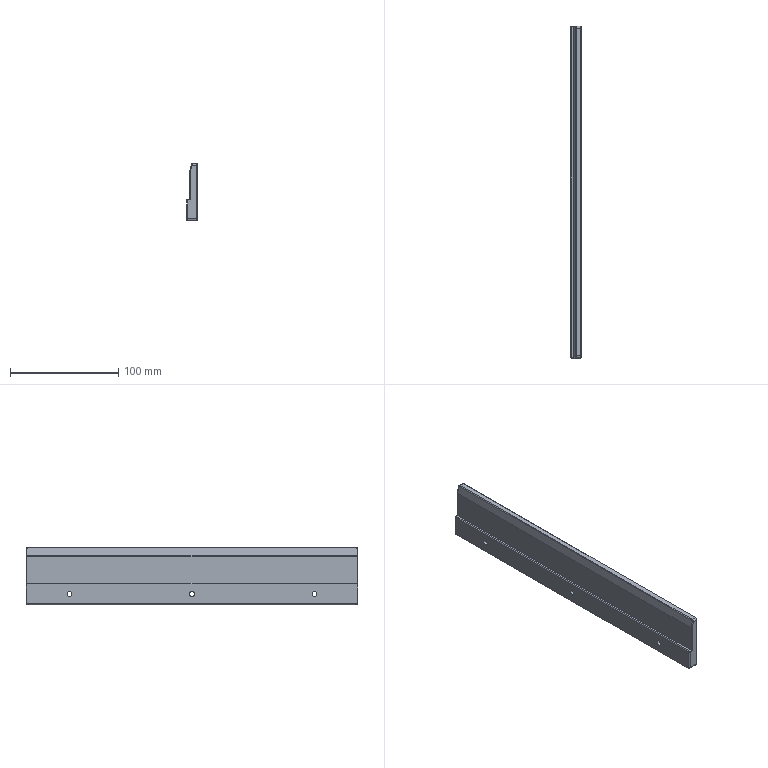Part | 1 solid | 53 faces | box 10 x 306 x 53 mm | volume 131374 mm3 | cylinder 22 | plane 16 | cone 7 | sphere 4 | spline 2 | torus 2 | commonest cylinder face diameters 1.5 x12 4 x4 4.5 x3 7.5 x3
STEP:
#1=CARTESIAN_POINT('',(315.5,-277.,153.));
#2=VERTEX_POINT('',#1);
#3=CARTESIAN_POINT('',(315.,-277.5,153.));
#4=VERTEX_POINT('',#3);
#5=CARTESIAN_POINT('',(315.5,-277.,153.));
#6=DIRECTION('',(-0.7071,-0.7071,0.));
#7=VECTOR('',#6,1000.);
#8=LINE('',#5,#7);
#9=EDGE_CURVE('',#2,#4,#8,.T.);
#10=ORIENTED_EDGE('',*,*,#9,.T.);
#11=CARTESIAN_POINT('',(315.,-275.5,151.));
#12=VERTEX_POINT('',#11);
#13=CARTESIAN_POINT('',(315.,-275.5,153.));
#14=DIRECTION('',(-1.,0.,0.));
#15=DIRECTION('',(0.,0.,-1.));
#16=AXIS2_PLACEMENT_3D('',#13,#14,#15);
#17=CIRCLE('',#16,2.);
#18=EDGE_CURVE('',#12,#4,#17,.T.);
#19=ORIENTED_EDGE('',*,*,#18,.F.);
#20=CARTESIAN_POINT('',(315.5,-275.5,151.5));
#21=VERTEX_POINT('',#20);
#22=CARTESIAN_POINT('',(315.,-275.5,151.));
#23=DIRECTION('',(0.7071,0.,0.7071));
#24=VECTOR('',#23,1000.);
#25=LINE('',#22,#24);
#26=EDGE_CURVE('',#12,#21,#25,.T.);
#27=ORIENTED_EDGE('',*,*,#26,.T.);
#28=CARTESIAN_POINT('',(315.5,-275.5,153.));
#29=DIRECTION('',(1.,0.,0.));
#30=DIRECTION('',(0.,0.,1.));
#31=AXIS2_PLACEMENT_3D('',#28,#29,#30);
#32=CIRCLE('',#31,1.5);
#33=EDGE_CURVE('',#2,#21,#32,.T.);
#34=ORIENTED_EDGE('',*,*,#33,.F.);
#35=EDGE_LOOP('',(#10,#19,#27,#34));
#36=FACE_BOUND('',#35,.T.);
#37=CARTESIAN_POINT('',(315.5,-275.5,153.));
#38=DIRECTION('',(-1.,0.,0.));
#39=DIRECTION('',(0.,0.,1.));
#40=AXIS2_PLACEMENT_3D('',#37,#38,#39);
#41=CONICAL_SURFACE('',#40,1.5,0.7854);
#42=ADVANCED_FACE('',(#36),#41,.T.);
#43=CARTESIAN_POINT('',(315.,26.5,151.));
#44=VERTEX_POINT('',#43);
#45=CARTESIAN_POINT('',(315.5,26.5,151.5));
#46=VERTEX_POINT('',#45);
#47=CARTESIAN_POINT('',(315.,26.5,151.));
#48=DIRECTION('',(0.7071,0.,0.7071));
#49=VECTOR('',#48,1000.);
#50=LINE('',#47,#49);
#51=EDGE_CURVE('',#44,#46,#50,.T.);
#52=ORIENTED_EDGE('',*,*,#51,.T.);
#53=CARTESIAN_POINT('',(315.5,26.5,151.5));
#54=DIRECTION('',(0.,1.,0.));
#55=VECTOR('',#54,1000.);
#56=LINE('',#53,#55);
#57=EDGE_CURVE('',#21,#46,#56,.T.);
#58=ORIENTED_EDGE('',*,*,#57,.F.);
#59=ORIENTED_EDGE('',*,*,#26,.F.);
#60=CARTESIAN_POINT('',(315.,-275.5,151.));
#61=DIRECTION('',(0.,-1.,0.));
#62=VECTOR('',#61,1000.);
#63=LINE('',#60,#62);
#64=EDGE_CURVE('',#44,#12,#63,.T.);
#65=ORIENTED_EDGE('',*,*,#64,.F.);
#66=EDGE_LOOP('',(#52,#58,#59,#65));
#67=FACE_BOUND('',#66,.T.);
#68=CARTESIAN_POINT('',(315.5,40.5,151.5));
#69=DIRECTION('',(-0.7071,0.,0.7071));
#70=DIRECTION('',(0.,1.,0.));
#71=AXIS2_PLACEMENT_3D('',#68,#69,#70);
#72=PLANE('',#71);
#73=ADVANCED_FACE('',(#67),#72,.F.);
#74=CARTESIAN_POINT('',(315.5,-277.,202.));
#75=VERTEX_POINT('',#74);
#76=CARTESIAN_POINT('',(315.,-277.5,202.));
#77=VERTEX_POINT('',#76);
#78=CARTESIAN_POINT('',(315.5,-277.,202.));
#79=DIRECTION('',(-0.7071,-0.7071,0.));
#80=VECTOR('',#79,1000.);
#81=LINE('',#78,#80);
#82=EDGE_CURVE('',#75,#77,#81,.T.);
#83=ORIENTED_EDGE('',*,*,#82,.T.);
#84=CARTESIAN_POINT('',(315.,-277.5,185.975));
#85=DIRECTION('',(0.,0.,1.));
#86=VECTOR('',#85,1000.);
#87=LINE('',#84,#86);
#88=EDGE_CURVE('',#4,#77,#87,.T.);
#89=ORIENTED_EDGE('',*,*,#88,.F.);
#90=ORIENTED_EDGE('',*,*,#9,.F.);
#91=CARTESIAN_POINT('',(315.5,-277.,193.));
#92=DIRECTION('',(0.,0.,-1.));
#93=VECTOR('',#92,1000.);
#94=LINE('',#91,#93);
#95=EDGE_CURVE('',#75,#2,#94,.T.);
#96=ORIENTED_EDGE('',*,*,#95,.F.);
#97=EDGE_LOOP('',(#83,#89,#90,#96));
#98=FACE_BOUND('',#97,.T.);
#99=CARTESIAN_POINT('',(315.,-277.5,185.975));
#100=DIRECTION('',(0.7071,-0.7071,0.));
#101=DIRECTION('',(0.,0.,-1.));
#102=AXIS2_PLACEMENT_3D('',#99,#100,#101);
#103=PLANE('',#102);
#104=ADVANCED_FACE('',(#98),#103,.T.);
#105=CARTESIAN_POINT('',(315.,28.5,153.));
#106=VERTEX_POINT('',#105);
#107=CARTESIAN_POINT('',(315.5,28.,153.));
#108=VERTEX_POINT('',#107);
#109=CARTESIAN_POINT('',(315.,28.5,153.));
#110=DIRECTION('',(0.7071,-0.7071,0.));
#111=VECTOR('',#110,1000.);
#112=LINE('',#109,#111);
#113=EDGE_CURVE('',#106,#108,#112,.T.);
#114=ORIENTED_EDGE('',*,*,#113,.T.);
#115=CARTESIAN_POINT('',(315.5,26.5,153.));
#116=DIRECTION('',(1.,0.,0.));
#117=DIRECTION('',(0.,0.,1.));
#118=AXIS2_PLACEMENT_3D('',#115,#116,#117);
#119=CIRCLE('',#118,1.5);
#120=EDGE_CURVE('',#46,#108,#119,.T.);
#121=ORIENTED_EDGE('',*,*,#120,.F.);
#122=ORIENTED_EDGE('',*,*,#51,.F.);
#123=CARTESIAN_POINT('',(315.,26.5,153.));
#124=DIRECTION('',(-1.,0.,0.));
#125=DIRECTION('',(0.,0.,-1.));
#126=AXIS2_PLACEMENT_3D('',#123,#124,#125);
#127=CIRCLE('',#126,2.);
#128=EDGE_CURVE('',#106,#44,#127,.T.);
#129=ORIENTED_EDGE('',*,*,#128,.F.);
#130=EDGE_LOOP('',(#114,#121,#122,#129));
#131=FACE_BOUND('',#130,.T.);
#132=CARTESIAN_POINT('',(315.5,26.5,153.));
#133=DIRECTION('',(-1.,0.,0.));
#134=DIRECTION('',(0.,0.,1.));
#135=AXIS2_PLACEMENT_3D('',#132,#133,#134);
#136=CONICAL_SURFACE('',#135,1.5,0.7854);
#137=ADVANCED_FACE('',(#131),#136,.T.);
#138=CARTESIAN_POINT('',(315.5,-275.5,203.5));
#139=VERTEX_POINT('',#138);
#140=CARTESIAN_POINT('',(315.,-275.5,204.));
#141=VERTEX_POINT('',#140);
#142=CARTESIAN_POINT('',(315.5,-275.5,203.5));
#143=DIRECTION('',(-0.7071,0.,0.7071));
#144=VECTOR('',#143,1000.);
#145=LINE('',#142,#144);
#146=EDGE_CURVE('',#139,#141,#145,.T.);
#147=ORIENTED_EDGE('',*,*,#146,.T.);
#148=CARTESIAN_POINT('',(315.,-275.5,202.));
#149=DIRECTION('',(-1.,0.,0.));
#150=DIRECTION('',(0.,0.,-1.));
#151=AXIS2_PLACEMENT_3D('',#148,#149,#150);
#152=CIRCLE('',#151,2.);
#153=EDGE_CURVE('',#77,#141,#152,.T.);
#154=ORIENTED_EDGE('',*,*,#153,.F.);
#155=ORIENTED_EDGE('',*,*,#82,.F.);
#156=CARTESIAN_POINT('',(315.5,-275.5,202.));
#157=DIRECTION('',(1.,0.,0.));
#158=DIRECTION('',(0.,0.,1.));
#159=AXIS2_PLACEMENT_3D('',#156,#157,#158);
#160=CIRCLE('',#159,1.5);
#161=EDGE_CURVE('',#139,#75,#160,.T.);
#162=ORIENTED_EDGE('',*,*,#161,.F.);
#163=EDGE_LOOP('',(#147,#154,#155,#162));
#164=FACE_BOUND('',#163,.T.);
#165=CARTESIAN_POINT('',(315.5,-275.5,202.));
#166=DIRECTION('',(-1.,0.,0.));
#167=DIRECTION('',(0.,0.,1.));
#168=AXIS2_PLACEMENT_3D('',#165,#166,#167);
#169=CONICAL_SURFACE('',#168,1.5,0.7854);
#170=ADVANCED_FACE('',(#164),#169,.T.);
#171=CARTESIAN_POINT('',(315.,28.5,202.));
#172=VERTEX_POINT('',#171);
#173=CARTESIAN_POINT('',(315.5,28.,202.));
#174=VERTEX_POINT('',#173);
#175=CARTESIAN_POINT('',(315.,28.5,202.));
#176=DIRECTION('',(0.7071,-0.7071,0.));
#177=VECTOR('',#176,1000.);
#178=LINE('',#175,#177);
#179=EDGE_CURVE('',#172,#174,#178,.T.);
#180=ORIENTED_EDGE('',*,*,#179,.T.);
#181=CARTESIAN_POINT('',(315.5,28.,193.));
#182=DIRECTION('',(0.,0.,1.));
#183=VECTOR('',#182,1000.);
#184=LINE('',#181,#183);
#185=EDGE_CURVE('',#108,#174,#184,.T.);
#186=ORIENTED_EDGE('',*,*,#185,.F.);
#187=ORIENTED_EDGE('',*,*,#113,.F.);
#188=CARTESIAN_POINT('',(315.,28.5,194.546));
#189=DIRECTION('',(0.,0.,-1.));
#190=VECTOR('',#189,1000.);
#191=LINE('',#188,#190);
#192=EDGE_CURVE('',#172,#106,#191,.T.);
#193=ORIENTED_EDGE('',*,*,#192,.F.);
#194=EDGE_LOOP('',(#180,#186,#187,#193));
#195=FACE_BOUND('',#194,.T.);
#196=CARTESIAN_POINT('',(315.5,28.,193.));
#197=DIRECTION('',(-0.7071,-0.7071,0.));
#198=DIRECTION('',(0.,0.,1.));
#199=AXIS2_PLACEMENT_3D('',#196,#197,#198);
#200=PLANE('',#199);
#201=ADVANCED_FACE('',(#195),#200,.F.);
#202=CARTESIAN_POINT('',(315.5,26.5,203.5));
#203=VERTEX_POINT('',#202);
#204=CARTESIAN_POINT('',(315.,26.5,204.));
#205=VERTEX_POINT('',#204);
#206=CARTESIAN_POINT('',(315.5,26.5,203.5));
#207=DIRECTION('',(-0.7071,0.,0.7071));
#208=VECTOR('',#207,1000.);
#209=LINE('',#206,#208);
#210=EDGE_CURVE('',#203,#205,#209,.T.);
#211=ORIENTED_EDGE('',*,*,#210,.T.);
#212=CARTESIAN_POINT('',(315.,26.5,204.));
#213=DIRECTION('',(0.,1.,0.));
#214=VECTOR('',#213,1000.);
#215=LINE('',#212,#214);
#216=EDGE_CURVE('',#141,#205,#215,.T.);
#217=ORIENTED_EDGE('',*,*,#216,.F.);
#218=ORIENTED_EDGE('',*,*,#146,.F.);
#219=CARTESIAN_POINT('',(315.5,-275.5,203.5));
#220=DIRECTION('',(0.,-1.,0.));
#221=VECTOR('',#220,1000.);
#222=LINE('',#219,#221);
#223=EDGE_CURVE('',#203,#139,#222,.T.);
#224=ORIENTED_EDGE('',*,*,#223,.F.);
#225=EDGE_LOOP('',(#211,#217,#218,#224));
#226=FACE_BOUND('',#225,.T.);
#227=CARTESIAN_POINT('',(315.5,40.5,203.5));
#228=DIRECTION('',(-0.7071,0.,-0.7071));
#229=DIRECTION('',(0.,-1.,0.));
#230=AXIS2_PLACEMENT_3D('',#227,#228,#229);
#231=PLANE('',#230);
#232=ADVANCED_FACE('',(#226),#231,.F.);
#233=ORIENTED_EDGE('',*,*,#179,.F.);
#234=CARTESIAN_POINT('',(315.,26.5,202.));
#235=DIRECTION('',(-1.,0.,0.));
#236=DIRECTION('',(0.,0.,-1.));
#237=AXIS2_PLACEMENT_3D('',#234,#235,#236);
#238=CIRCLE('',#237,2.);
#239=EDGE_CURVE('',#205,#172,#238,.T.);
#240=ORIENTED_EDGE('',*,*,#239,.F.);
#241=ORIENTED_EDGE('',*,*,#210,.F.);
#242=CARTESIAN_POINT('',(315.5,26.5,202.));
#243=DIRECTION('',(1.,0.,0.));
#244=DIRECTION('',(0.,0.,1.));
#245=AXIS2_PLACEMENT_3D('',#242,#243,#244);
#246=CIRCLE('',#245,1.5);
#247=EDGE_CURVE('',#174,#203,#246,.T.);
#248=ORIENTED_EDGE('',*,*,#247,.F.);
#249=EDGE_LOOP('',(#233,#240,#241,#248));
#250=FACE_BOUND('',#249,.T.);
#251=CARTESIAN_POINT('',(315.5,26.5,202.));
#252=DIRECTION('',(-1.,0.,0.));
#253=DIRECTION('',(0.,0.,1.));
#254=AXIS2_PLACEMENT_3D('',#251,#252,#253);
#255=CONICAL_SURFACE('',#254,1.5,0.7854);
#256=ADVANCED_FACE('',(#250),#255,.T.);
#257=CARTESIAN_POINT('',(308.2,27.75,171.));
#258=VERTEX_POINT('',#257);
#259=CARTESIAN_POINT('',(308.95,28.5,170.25));
#260=VERTEX_POINT('',#259);
#261=CARTESIAN_POINT('',(308.95,27.75,170.25));
#262=DIRECTION('',(-0.7071,0.,-0.7071));
#263=DIRECTION('',(0.7071,0.,-0.7071));
#264=AXIS2_PLACEMENT_3D('',#261,#262,#263);
#265=ELLIPSE('',#264,1.061,0.75);
#266=EDGE_CURVE('',#258,#260,#265,.T.);
#267=ORIENTED_EDGE('',*,*,#266,.F.);
#268=CARTESIAN_POINT('',(308.2,27.75,195.908));
#269=VERTEX_POINT('',#268);
#270=CARTESIAN_POINT('',(308.2,27.75,193.));
#271=DIRECTION('',(0.,0.,-1.));
#272=VECTOR('',#271,1000.);
#273=LINE('',#270,#272);
#274=EDGE_CURVE('',#269,#258,#273,.T.);
#275=ORIENTED_EDGE('',*,*,#274,.F.);
#276=CARTESIAN_POINT('',(308.95,28.5,195.908));
#277=VERTEX_POINT('',#276);
#278=CARTESIAN_POINT('',(308.95,27.75,195.908));
#279=DIRECTION('',(0.,0.,-1.));
#280=DIRECTION('',(-1.,0.,0.));
#281=AXIS2_PLACEMENT_3D('',#278,#279,#280);
#282=CIRCLE('',#281,0.75);
#283=EDGE_CURVE('',#269,#277,#282,.T.);
#284=ORIENTED_EDGE('',*,*,#283,.T.);
#285=CARTESIAN_POINT('',(308.95,28.5,194.546));
#286=DIRECTION('',(0.,0.,1.));
#287=VECTOR('',#286,1000.);
#288=LINE('',#285,#287);
#289=EDGE_CURVE('',#260,#277,#288,.T.);
#290=ORIENTED_EDGE('',*,*,#289,.F.);
#291=EDGE_LOOP('',(#267,#275,#284,#290));
#292=FACE_BOUND('',#291,.T.);
#293=CARTESIAN_POINT('',(308.95,27.75,194.546));
#294=DIRECTION('',(0.,0.,-1.));
#295=DIRECTION('',(-1.,0.,0.));
#296=AXIS2_PLACEMENT_3D('',#293,#294,#295);
#297=CYLINDRICAL_SURFACE('',#296,0.75);
#298=ADVANCED_FACE('',(#292),#297,.T.);
#299=CARTESIAN_POINT('',(308.222,27.75,196.09));
#300=VERTEX_POINT('',#299);
#301=CARTESIAN_POINT('',(308.95,27.75,195.908));
#302=DIRECTION('',(0.,1.,0.));
#303=DIRECTION('',(0.,0.,1.));
#304=AXIS2_PLACEMENT_3D('',#301,#302,#303);
#305=CIRCLE('',#304,0.75);
#306=EDGE_CURVE('',#269,#300,#305,.T.);
#307=ORIENTED_EDGE('',*,*,#306,.T.);
#308=CARTESIAN_POINT('',(308.95,27.75,195.908));
#309=DIRECTION('',(-0.2425,0.,-0.9701));
#310=DIRECTION('',(-0.9701,0.,0.2425));
#311=AXIS2_PLACEMENT_3D('',#308,#309,#310);
#312=CIRCLE('',#311,0.75);
#313=EDGE_CURVE('',#300,#277,#312,.T.);
#314=ORIENTED_EDGE('',*,*,#313,.T.);
#315=ORIENTED_EDGE('',*,*,#283,.F.);
#316=EDGE_LOOP('',(#307,#314,#315));
#317=FACE_BOUND('',#316,.T.);
#318=CARTESIAN_POINT('',(308.95,27.75,195.908));
#319=DIRECTION('',(0.,0.,1.));
#320=DIRECTION('',(1.,0.,0.));
#321=AXIS2_PLACEMENT_3D('',#318,#319,#320);
#322=SPHERICAL_SURFACE('',#321,0.75);
#323=ADVANCED_FACE('',(#317),#322,.T.);
#324=CARTESIAN_POINT('',(308.2,-276.75,195.908));
#325=VERTEX_POINT('',#324);
#326=CARTESIAN_POINT('',(308.222,-276.75,196.09));
#327=VERTEX_POINT('',#326);
#328=CARTESIAN_POINT('',(308.95,-276.75,195.908));
#329=DIRECTION('',(0.,1.,0.));
#330=DIRECTION('',(0.,0.,1.));
#331=AXIS2_PLACEMENT_3D('',#328,#329,#330);
#332=CIRCLE('',#331,0.75);
#333=EDGE_CURVE('',#325,#327,#332,.T.);
#334=ORIENTED_EDGE('',*,*,#333,.T.);
#335=CARTESIAN_POINT('',(308.222,-124.,196.09));
#336=DIRECTION('',(0.,-1.,0.));
#337=VECTOR('',#336,1000.);
#338=LINE('',#335,#337);
#339=EDGE_CURVE('',#300,#327,#338,.T.);
#340=ORIENTED_EDGE('',*,*,#339,.F.);
#341=ORIENTED_EDGE('',*,*,#306,.F.);
#342=CARTESIAN_POINT('',(308.2,40.5,195.908));
#343=DIRECTION('',(0.,1.,0.));
#344=VECTOR('',#343,1000.);
#345=LINE('',#342,#344);
#346=EDGE_CURVE('',#325,#269,#345,.T.);
#347=ORIENTED_EDGE('',*,*,#346,.F.);
#348=EDGE_LOOP('',(#334,#340,#341,#347));
#349=FACE_BOUND('',#348,.T.);
#350=CARTESIAN_POINT('',(308.95,40.5,195.908));
#351=DIRECTION('',(0.,1.,0.));
#352=DIRECTION('',(0.,0.,1.));
#353=AXIS2_PLACEMENT_3D('',#350,#351,#352);
#354=CYLINDRICAL_SURFACE('',#353,0.75);
#355=ADVANCED_FACE('',(#349),#354,.T.);
#356=CARTESIAN_POINT('',(309.745,27.75,202.182));
#357=VERTEX_POINT('',#356);
#358=CARTESIAN_POINT('',(310.473,28.5,202.));
#359=VERTEX_POINT('',#358);
#360=CARTESIAN_POINT('',(310.473,27.75,202.));
#361=DIRECTION('',(0.2425,0.,0.9701));
#362=DIRECTION('',(0.9701,0.,-0.2425));
#363=AXIS2_PLACEMENT_3D('',#360,#361,#362);
#364=CIRCLE('',#363,0.75);
#365=EDGE_CURVE('',#357,#359,#364,.F.);
#366=ORIENTED_EDGE('',*,*,#365,.T.);
#367=CARTESIAN_POINT('',(305.669,28.5,182.785));
#368=DIRECTION('',(0.2425,0.,0.9701));
#369=VECTOR('',#368,1000.);
#370=LINE('',#367,#369);
#371=EDGE_CURVE('',#277,#359,#370,.T.);
#372=ORIENTED_EDGE('',*,*,#371,.F.);
#373=ORIENTED_EDGE('',*,*,#313,.F.);
#374=CARTESIAN_POINT('',(310.2,27.75,204.));
#375=DIRECTION('',(-0.2425,0.,-0.9701));
#376=VECTOR('',#375,1000.);
#377=LINE('',#374,#376);
#378=EDGE_CURVE('',#357,#300,#377,.T.);
#379=ORIENTED_EDGE('',*,*,#378,.F.);
#380=EDGE_LOOP('',(#366,#372,#373,#379));
#381=FACE_BOUND('',#380,.T.);
#382=CARTESIAN_POINT('',(305.669,27.75,182.785));
#383=DIRECTION('',(-0.2425,0.,-0.9701));
#384=DIRECTION('',(-0.9701,0.,0.2425));
#385=AXIS2_PLACEMENT_3D('',#382,#383,#384);
#386=CYLINDRICAL_SURFACE('',#385,0.75);
#387=ADVANCED_FACE('',(#381),#386,.T.);
#388=CARTESIAN_POINT('',(308.95,-277.5,195.908));
#389=VERTEX_POINT('',#388);
#390=CARTESIAN_POINT('',(308.95,-276.75,195.908));
#391=DIRECTION('',(0.,0.,-1.));
#392=DIRECTION('',(-1.,0.,0.));
#393=AXIS2_PLACEMENT_3D('',#390,#391,#392);
#394=CIRCLE('',#393,0.75);
#395=EDGE_CURVE('',#325,#389,#394,.F.);
#396=ORIENTED_EDGE('',*,*,#395,.T.);
#397=CARTESIAN_POINT('',(308.95,-276.75,195.908));
#398=DIRECTION('',(-0.2425,0.,-0.9701));
#399=DIRECTION('',(-0.9701,0.,0.2425));
#400=AXIS2_PLACEMENT_3D('',#397,#398,#399);
#401=CIRCLE('',#400,0.75);
#402=EDGE_CURVE('',#389,#327,#401,.T.);
#403=ORIENTED_EDGE('',*,*,#402,.T.);
#404=ORIENTED_EDGE('',*,*,#333,.F.);
#405=EDGE_LOOP('',(#396,#403,#404));
#406=FACE_BOUND('',#405,.T.);
#407=CARTESIAN_POINT('',(308.95,-276.75,195.908));
#408=DIRECTION('',(0.,0.,1.));
#409=DIRECTION('',(1.,0.,0.));
#410=AXIS2_PLACEMENT_3D('',#407,#408,#409);
#411=SPHERICAL_SURFACE('',#410,0.75);
#412=ADVANCED_FACE('',(#406),#411,.T.);
#413=CARTESIAN_POINT('',(310.058,26.5,203.432));
#414=VERTEX_POINT('',#413);
#415=CARTESIAN_POINT('',(310.786,26.5,204.));
#416=VERTEX_POINT('',#415);
#417=CARTESIAN_POINT('',(310.786,26.5,203.25));
#418=DIRECTION('',(0.,1.,0.));
#419=DIRECTION('',(0.,0.,1.));
#420=AXIS2_PLACEMENT_3D('',#417,#418,#419);
#421=CIRCLE('',#420,0.75);
#422=EDGE_CURVE('',#414,#416,#421,.T.);
#423=ORIENTED_EDGE('',*,*,#422,.T.);
#424=CARTESIAN_POINT('',(310.473,26.5,202.));
#425=DIRECTION('',(0.988,0.,-0.1544));
#426=DIRECTION('',(0.1544,0.,0.988));
#427=AXIS2_PLACEMENT_3D('',#424,#425,#426);
#428=ELLIPSE('',#427,2.024,2.);
#429=EDGE_CURVE('',#359,#416,#428,.T.);
#430=ORIENTED_EDGE('',*,*,#429,.F.);
#431=ORIENTED_EDGE('',*,*,#365,.F.);
#432=CARTESIAN_POINT('',(309.745,26.5,202.182));
#433=DIRECTION('',(-0.9701,0.,0.2425));
#434=DIRECTION('',(0.2425,0.,0.9701));
#435=AXIS2_PLACEMENT_3D('',#432,#433,#434);
#436=ELLIPSE('',#435,1.288,1.25);
#437=EDGE_CURVE('',#414,#357,#436,.T.);
#438=ORIENTED_EDGE('',*,*,#437,.F.);
#439=EDGE_LOOP('',(#423,#430,#431,#438));
#440=FACE_BOUND('',#439,.T.);
#441=CARTESIAN_POINT('',(310.786,26.5,204.));
#442=CARTESIAN_POINT('',(310.2,26.5,204.));
#443=CARTESIAN_POINT('',(310.058,26.5,203.432));
#444=CARTESIAN_POINT('',(310.786,27.024,204.));
#445=CARTESIAN_POINT('',(310.2,26.985,204.));
#446=CARTESIAN_POINT('',(310.058,26.827,203.432));
#447=CARTESIAN_POINT('',(310.718,28.067,203.567));
#448=CARTESIAN_POINT('',(310.104,27.98,203.617));
#449=CARTESIAN_POINT('',(309.99,27.479,203.161));
#450=CARTESIAN_POINT('',(310.555,28.5,202.524));
#451=CARTESIAN_POINT('',(309.87,28.454,202.678));
#452=CARTESIAN_POINT('',(309.827,27.75,202.509));
#453=CARTESIAN_POINT('',(310.473,28.5,202.));
#454=CARTESIAN_POINT('',(309.745,28.5,202.182));
#455=CARTESIAN_POINT('',(309.745,27.75,202.182));
#456=(BOUNDED_SURFACE()B_SPLINE_SURFACE(3,2,((#441,#442,#443),(#444,#445,#446),(#447,#448,#449),(#450,#451,#452),(#453,#454,#455)),.UNSPECIFIED.,.F.,.F.,.F.)B_SPLINE_SURFACE_WITH_KNOTS((4,1,4),(3,3),(0.,0.7854,1.571),(0.,1.),.UNSPECIFIED.)GEOMETRIC_REPRESENTATION_ITEM()RATIONAL_B_SPLINE_SURFACE(((1.,0.7882,1.),(1.,0.7882,1.),(1.,0.7718,1.),(1.,0.7296,1.),(1.,0.7071,1.)))REPRESENTATION_ITEM('')SURFACE());
#457=ADVANCED_FACE('',(#440),#456,.T.);
#458=CARTESIAN_POINT('',(308.95,-277.5,170.25));
#459=VERTEX_POINT('',#458);
#460=CARTESIAN_POINT('',(308.2,-276.75,171.));
#461=VERTEX_POINT('',#460);
#462=CARTESIAN_POINT('',(308.95,-276.75,170.25));
#463=DIRECTION('',(-0.7071,0.,-0.7071));
#464=DIRECTION('',(0.7071,0.,-0.7071));
#465=AXIS2_PLACEMENT_3D('',#462,#463,#464);
#466=ELLIPSE('',#465,1.061,0.75);
#467=EDGE_CURVE('',#459,#461,#466,.T.);
#468=ORIENTED_EDGE('',*,*,#467,.F.);
#469=CARTESIAN_POINT('',(308.95,-277.5,185.975));
#470=DIRECTION('',(0.,0.,-1.));
#471=VECTOR('',#470,1000.);
#472=LINE('',#469,#471);
#473=EDGE_CURVE('',#389,#459,#472,.T.);
#474=ORIENTED_EDGE('',*,*,#473,.F.);
#475=ORIENTED_EDGE('',*,*,#395,.F.);
#476=CARTESIAN_POINT('',(308.2,-276.75,193.));
#477=DIRECTION('',(0.,0.,1.));
#478=VECTOR('',#477,1000.);
#479=LINE('',#476,#478);
#480=EDGE_CURVE('',#461,#325,#479,.T.);
#481=ORIENTED_EDGE('',*,*,#480,.F.);
#482=EDGE_LOOP('',(#468,#474,#475,#481));
#483=FACE_BOUND('',#482,.T.);
#484=CARTESIAN_POINT('',(308.95,-276.75,185.975));
#485=DIRECTION('',(0.,0.,-1.));
#486=DIRECTION('',(-1.,0.,0.));
#487=AXIS2_PLACEMENT_3D('',#484,#485,#486);
#488=CYLINDRICAL_SURFACE('',#487,0.75);
#489=ADVANCED_FACE('',(#483),#488,.T.);
#490=CARTESIAN_POINT('',(310.473,-277.5,202.));
#491=VERTEX_POINT('',#490);
#492=CARTESIAN_POINT('',(309.745,-276.75,202.182));
#493=VERTEX_POINT('',#492);
#494=CARTESIAN_POINT('',(310.473,-276.75,202.));
#495=DIRECTION('',(-0.2425,0.,-0.9701));
#496=DIRECTION('',(-0.9701,0.,0.2425));
#497=AXIS2_PLACEMENT_3D('',#494,#495,#496);
#498=CIRCLE('',#497,0.75);
#499=EDGE_CURVE('',#491,#493,#498,.T.);
#500=ORIENTED_EDGE('',*,*,#499,.T.);
#501=CARTESIAN_POINT('',(310.2,-276.75,204.));
#502=DIRECTION('',(0.2425,0.,0.9701));
#503=VECTOR('',#502,1000.);
#504=LINE('',#501,#503);
#505=EDGE_CURVE('',#327,#493,#504,.T.);
#506=ORIENTED_EDGE('',*,*,#505,.F.);
#507=ORIENTED_EDGE('',*,*,#402,.F.);
#508=CARTESIAN_POINT('',(303.498,-277.5,174.101));
#509=DIRECTION('',(-0.2425,0.,-0.9701));
#510=VECTOR('',#509,1000.);
#511=LINE('',#508,#510);
#512=EDGE_CURVE('',#491,#389,#511,.T.);
#513=ORIENTED_EDGE('',*,*,#512,.F.);
#514=EDGE_LOOP('',(#500,#506,#507,#513));
#515=FACE_BOUND('',#514,.T.);
#516=CARTESIAN_POINT('',(303.498,-276.75,174.101));
#517=DIRECTION('',(-0.2425,0.,-0.9701));
#518=DIRECTION('',(-0.9701,0.,0.2425));
#519=AXIS2_PLACEMENT_3D('',#516,#517,#518);
#520=CYLINDRICAL_SURFACE('',#519,0.75);
#521=ADVANCED_FACE('',(#515),#520,.T.);
#522=CARTESIAN_POINT('',(310.058,-275.5,203.432));
#523=VERTEX_POINT('',#522);
#524=CARTESIAN_POINT('',(310.786,-275.5,204.));
#525=VERTEX_POINT('',#524);
#526=CARTESIAN_POINT('',(310.786,-275.5,203.25));
#527=DIRECTION('',(0.,-1.,0.));
#528=DIRECTION('',(0.,0.,-1.));
#529=AXIS2_PLACEMENT_3D('',#526,#527,#528);
#530=CIRCLE('',#529,0.75);
#531=EDGE_CURVE('',#523,#525,#530,.F.);
#532=ORIENTED_EDGE('',*,*,#531,.T.);
#533=CARTESIAN_POINT('',(310.786,-275.5,204.));
#534=DIRECTION('',(0.,-1.,0.));
#535=VECTOR('',#534,1000.);
#536=LINE('',#533,#535);
#537=EDGE_CURVE('',#416,#525,#536,.T.);
#538=ORIENTED_EDGE('',*,*,#537,.F.);
#539=ORIENTED_EDGE('',*,*,#422,.F.);
#540=CARTESIAN_POINT('',(310.058,26.5,203.432));
#541=DIRECTION('',(0.,1.,0.));
#542=VECTOR('',#541,1000.);
#543=LINE('',#540,#542);
#544=EDGE_CURVE('',#523,#414,#543,.T.);
#545=ORIENTED_EDGE('',*,*,#544,.F.);
#546=EDGE_LOOP('',(#532,#538,#539,#545));
#547=FACE_BOUND('',#546,.T.);
#548=CARTESIAN_POINT('',(310.786,-124.,203.25));
#549=DIRECTION('',(0.,1.,0.));
#550=DIRECTION('',(0.,0.,1.));
#551=AXIS2_PLACEMENT_3D('',#548,#549,#550);
#552=CYLINDRICAL_SURFACE('',#551,0.75);
#553=ADVANCED_FACE('',(#547),#552,.T.);
#554=ORIENTED_EDGE('',*,*,#499,.F.);
#555=CARTESIAN_POINT('',(310.473,-275.5,202.));
#556=DIRECTION('',(0.988,0.,-0.1544));
#557=DIRECTION('',(0.1544,0.,0.988));
#558=AXIS2_PLACEMENT_3D('',#555,#556,#557);
#559=ELLIPSE('',#558,2.024,2.);
#560=EDGE_CURVE('',#525,#491,#559,.T.);
#561=ORIENTED_EDGE('',*,*,#560,.F.);
#562=ORIENTED_EDGE('',*,*,#531,.F.);
#563=CARTESIAN_POINT('',(309.745,-275.5,202.182));
#564=DIRECTION('',(-0.9701,0.,0.2425));
#565=DIRECTION('',(0.2425,0.,0.9701));
#566=AXIS2_PLACEMENT_3D('',#563,#564,#565);
#567=ELLIPSE('',#566,1.288,1.25);
#568=EDGE_CURVE('',#493,#523,#567,.T.);
#569=ORIENTED_EDGE('',*,*,#568,.F.);
#570=EDGE_LOOP('',(#554,#561,#562,#569));
#571=FACE_BOUND('',#570,.T.);
#572=CARTESIAN_POINT('',(310.473,-277.5,202.));
#573=CARTESIAN_POINT('',(309.745,-277.5,202.182));
#574=CARTESIAN_POINT('',(309.745,-276.75,202.182));
#575=CARTESIAN_POINT('',(310.555,-277.5,202.524));
#576=CARTESIAN_POINT('',(309.87,-277.454,202.678));
#577=CARTESIAN_POINT('',(309.827,-276.75,202.509));
#578=CARTESIAN_POINT('',(310.718,-277.067,203.567));
#579=CARTESIAN_POINT('',(310.104,-276.98,203.617));
#580=CARTESIAN_POINT('',(309.99,-276.479,203.161));
#581=CARTESIAN_POINT('',(310.786,-276.024,204.));
#582=CARTESIAN_POINT('',(310.2,-275.985,204.));
#583=CARTESIAN_POINT('',(310.058,-275.827,203.432));
#584=CARTESIAN_POINT('',(310.786,-275.5,204.));
#585=CARTESIAN_POINT('',(310.2,-275.5,204.));
#586=CARTESIAN_POINT('',(310.058,-275.5,203.432));
#587=(BOUNDED_SURFACE()B_SPLINE_SURFACE(3,2,((#572,#573,#574),(#575,#576,#577),(#578,#579,#580),(#581,#582,#583),(#584,#585,#586)),.UNSPECIFIED.,.F.,.F.,.F.)B_SPLINE_SURFACE_WITH_KNOTS((4,1,4),(3,3),(4.712,5.498,6.283),(0.,1.),.UNSPECIFIED.)GEOMETRIC_REPRESENTATION_ITEM()RATIONAL_B_SPLINE_SURFACE(((1.,0.7071,1.),(1.,0.7296,1.),(1.,0.7718,1.),(1.,0.7882,1.),(1.,0.7882,1.)))REPRESENTATION_ITEM('')SURFACE());
#588=ADVANCED_FACE('',(#571),#587,.T.);
#589=CARTESIAN_POINT('',(306.25,-277.5,170.25));
#590=VERTEX_POINT('',#589);
#591=CARTESIAN_POINT('',(305.5,-276.75,170.25));
#592=VERTEX_POINT('',#591);
#593=CARTESIAN_POINT('',(306.25,-276.75,170.25));
#594=DIRECTION('',(0.,0.,-1.));
#595=DIRECTION('',(-1.,0.,0.));
#596=AXIS2_PLACEMENT_3D('',#593,#594,#595);
#597=CIRCLE('',#596,0.75);
#598=EDGE_CURVE('',#590,#592,#597,.T.);
#599=ORIENTED_EDGE('',*,*,#598,.T.);
#600=CARTESIAN_POINT('',(305.5,-276.75,153.));
#601=VERTEX_POINT('',#600);
#602=CARTESIAN_POINT('',(305.5,-276.75,140.5));
#603=DIRECTION('',(0.,0.,1.));
#604=VECTOR('',#603,1000.);
#605=LINE('',#602,#604);
#606=EDGE_CURVE('',#601,#592,#605,.T.);
#607=ORIENTED_EDGE('',*,*,#606,.F.);
#608=CARTESIAN_POINT('',(306.25,-277.5,153.));
#609=VERTEX_POINT('',#608);
#610=CARTESIAN_POINT('',(306.25,-276.75,153.));
#611=DIRECTION('',(0.,0.,1.));
#612=DIRECTION('',(1.,0.,0.));
#613=AXIS2_PLACEMENT_3D('',#610,#611,#612);
#614=CIRCLE('',#613,0.75);
#615=EDGE_CURVE('',#601,#609,#614,.T.);
#616=ORIENTED_EDGE('',*,*,#615,.T.);
#617=CARTESIAN_POINT('',(306.25,-277.5,185.975));
#618=DIRECTION('',(0.,0.,-1.));
#619=VECTOR('',#618,1000.);
#620=LINE('',#617,#619);
#621=EDGE_CURVE('',#590,#609,#620,.T.);
#622=ORIENTED_EDGE('',*,*,#621,.F.);
#623=EDGE_LOOP('',(#599,#607,#616,#622));
#624=FACE_BOUND('',#623,.T.);
#625=CARTESIAN_POINT('',(306.25,-276.75,185.975));
#626=DIRECTION('',(0.,0.,-1.));
#627=DIRECTION('',(-1.,0.,0.));
#628=AXIS2_PLACEMENT_3D('',#625,#626,#627);
#629=CYLINDRICAL_SURFACE('',#628,0.75);
#630=ADVANCED_FACE('',(#624),#629,.T.);
#631=CARTESIAN_POINT('',(305.5,-275.5,151.75));
#632=VERTEX_POINT('',#631);
#633=CARTESIAN_POINT('',(306.25,-275.5,151.));
#634=VERTEX_POINT('',#633);
#635=CARTESIAN_POINT('',(306.25,-275.5,151.75));
#636=DIRECTION('',(0.,-1.,0.));
#637=DIRECTION('',(0.,0.,-1.));
#638=AXIS2_PLACEMENT_3D('',#635,#636,#637);
#639=CIRCLE('',#638,0.75);
#640=EDGE_CURVE('',#632,#634,#639,.T.);
#641=ORIENTED_EDGE('',*,*,#640,.T.);
#642=CARTESIAN_POINT('',(306.25,-275.5,153.));
#643=DIRECTION('',(1.,0.,0.));
#644=DIRECTION('',(0.,0.,1.));
#645=AXIS2_PLACEMENT_3D('',#642,#643,#644);
#646=CIRCLE('',#645,2.);
#647=EDGE_CURVE('',#609,#634,#646,.T.);
#648=ORIENTED_EDGE('',*,*,#647,.F.);
#649=ORIENTED_EDGE('',*,*,#615,.F.);
#650=CARTESIAN_POINT('',(305.5,-275.5,153.));
#651=DIRECTION('',(-1.,0.,0.));
#652=DIRECTION('',(0.,0.,1.));
#653=AXIS2_PLACEMENT_3D('',#650,#651,#652);
#654=CIRCLE('',#653,1.25);
#655=EDGE_CURVE('',#632,#601,#654,.T.);
#656=ORIENTED_EDGE('',*,*,#655,.F.);
#657=EDGE_LOOP('',(#641,#648,#649,#656));
#658=FACE_BOUND('',#657,.T.);
#659=CARTESIAN_POINT('',(306.25,-275.5,153.));
#660=DIRECTION('',(-1.,0.,0.));
#661=DIRECTION('',(0.,0.,1.));
#662=AXIS2_PLACEMENT_3D('',#659,#660,#661);
#663=TOROIDAL_SURFACE('',#662,1.25,0.75);
#664=ADVANCED_FACE('',(#658),#663,.T.);
#665=CARTESIAN_POINT('',(306.25,-276.75,171.));
#666=VERTEX_POINT('',#665);
#667=CARTESIAN_POINT('',(306.25,-276.75,170.25));
#668=DIRECTION('',(1.,0.,0.));
#669=DIRECTION('',(0.,0.,-1.));
#670=AXIS2_PLACEMENT_3D('',#667,#668,#669);
#671=CIRCLE('',#670,0.75);
#672=EDGE_CURVE('',#590,#666,#671,.F.);
#673=ORIENTED_EDGE('',*,*,#672,.T.);
#674=CARTESIAN_POINT('',(306.25,-276.75,170.25));
#675=DIRECTION('',(0.,1.,0.));
#676=DIRECTION('',(-1.,0.,0.));
#677=AXIS2_PLACEMENT_3D('',#674,#675,#676);
#678=CIRCLE('',#677,0.75);
#679=EDGE_CURVE('',#666,#592,#678,.F.);
#680=ORIENTED_EDGE('',*,*,#679,.T.);
#681=ORIENTED_EDGE('',*,*,#598,.F.);
#682=EDGE_LOOP('',(#673,#680,#681));
#683=FACE_BOUND('',#682,.T.);
#684=CARTESIAN_POINT('',(306.25,-276.75,170.25));
#685=DIRECTION('',(0.,0.,1.));
#686=DIRECTION('',(1.,0.,0.));
#687=AXIS2_PLACEMENT_3D('',#684,#685,#686);
#688=SPHERICAL_SURFACE('',#687,0.75);
#689=ADVANCED_FACE('',(#683),#688,.T.);
#690=CARTESIAN_POINT('',(305.5,26.5,151.75));
#691=VERTEX_POINT('',#690);
#692=CARTESIAN_POINT('',(306.25,26.5,151.));
#693=VERTEX_POINT('',#692);
#694=CARTESIAN_POINT('',(306.25,26.5,151.75));
#695=DIRECTION('',(0.,-1.,0.));
#696=DIRECTION('',(0.,0.,-1.));
#697=AXIS2_PLACEMENT_3D('',#694,#695,#696);
#698=CIRCLE('',#697,0.75);
#699=EDGE_CURVE('',#691,#693,#698,.T.);
#700=ORIENTED_EDGE('',*,*,#699,.T.);
#701=CARTESIAN_POINT('',(306.25,26.5,151.));
#702=DIRECTION('',(0.,1.,0.));
#703=VECTOR('',#702,1000.);
#704=LINE('',#701,#703);
#705=EDGE_CURVE('',#634,#693,#704,.T.);
#706=ORIENTED_EDGE('',*,*,#705,.F.);
#707=ORIENTED_EDGE('',*,*,#640,.F.);
#708=CARTESIAN_POINT('',(305.5,-275.5,151.75));
#709=DIRECTION('',(0.,-1.,0.));
#710=VECTOR('',#709,1000.);
#711=LINE('',#708,#710);
#712=EDGE_CURVE('',#691,#632,#711,.T.);
#713=ORIENTED_EDGE('',*,*,#712,.F.);
#714=EDGE_LOOP('',(#700,#706,#707,#713));
#715=FACE_BOUND('',#714,.T.);
#716=CARTESIAN_POINT('',(306.25,-105.,151.75));
#717=DIRECTION('',(0.,-1.,0.));
#718=DIRECTION('',(1.,0.,0.));
#719=AXIS2_PLACEMENT_3D('',#716,#717,#718);
#720=CYLINDRICAL_SURFACE('',#719,0.75);
#721=ADVANCED_FACE('',(#715),#720,.T.);
#722=CARTESIAN_POINT('',(256.,-277.5,170.25));
#723=DIRECTION('',(-1.,0.,0.));
#724=VECTOR('',#723,1000.);
#725=LINE('',#722,#724);
#726=EDGE_CURVE('',#459,#590,#725,.T.);
#727=ORIENTED_EDGE('',*,*,#726,.F.);
#728=ORIENTED_EDGE('',*,*,#467,.T.);
#729=CARTESIAN_POINT('',(296.,-276.75,171.));
#730=DIRECTION('',(1.,0.,0.));
#731=VECTOR('',#730,1000.);
#732=LINE('',#729,#731);
#733=EDGE_CURVE('',#666,#461,#732,.T.);
#734=ORIENTED_EDGE('',*,*,#733,.F.);
#735=ORIENTED_EDGE('',*,*,#672,.F.);
#736=EDGE_LOOP('',(#727,#728,#734,#735));
#737=FACE_BOUND('',#736,.T.);
#738=CARTESIAN_POINT('',(296.,-276.75,170.25));
#739=DIRECTION('',(1.,0.,0.));
#740=DIRECTION('',(0.,0.,-1.));
#741=AXIS2_PLACEMENT_3D('',#738,#739,#740);
#742=CYLINDRICAL_SURFACE('',#741,0.75);
#743=ADVANCED_FACE('',(#737),#742,.T.);
#744=CARTESIAN_POINT('',(306.25,27.75,171.));
#745=VERTEX_POINT('',#744);
#746=CARTESIAN_POINT('',(305.5,27.75,170.25));
#747=VERTEX_POINT('',#746);
#748=CARTESIAN_POINT('',(306.25,27.75,170.25));
#749=DIRECTION('',(0.,1.,0.));
#750=DIRECTION('',(-1.,0.,0.));
#751=AXIS2_PLACEMENT_3D('',#748,#749,#750);
#752=CIRCLE('',#751,0.75);
#753=EDGE_CURVE('',#745,#747,#752,.F.);
#754=ORIENTED_EDGE('',*,*,#753,.T.);
#755=CARTESIAN_POINT('',(305.5,-5.,170.25));
#756=DIRECTION('',(0.,1.,0.));
#757=VECTOR('',#756,1000.);
#758=LINE('',#755,#757);
#759=EDGE_CURVE('',#592,#747,#758,.T.);
#760=ORIENTED_EDGE('',*,*,#759,.F.);
#761=ORIENTED_EDGE('',*,*,#679,.F.);
#762=CARTESIAN_POINT('',(306.25,-105.,171.));
#763=DIRECTION('',(0.,-1.,0.));
#764=VECTOR('',#763,1000.);
#765=LINE('',#762,#764);
#766=EDGE_CURVE('',#745,#666,#765,.T.);
#767=ORIENTED_EDGE('',*,*,#766,.F.);
#768=EDGE_LOOP('',(#754,#760,#761,#767));
#769=FACE_BOUND('',#768,.T.);
#770=CARTESIAN_POINT('',(306.25,-5.,170.25));
#771=DIRECTION('',(0.,1.,0.));
#772=DIRECTION('',(-1.,0.,0.));
#773=AXIS2_PLACEMENT_3D('',#770,#771,#772);
#774=CYLINDRICAL_SURFACE('',#773,0.75);
#775=ADVANCED_FACE('',(#769),#774,.T.);
#776=CARTESIAN_POINT('',(305.5,27.75,153.));
#777=VERTEX_POINT('',#776);
#778=CARTESIAN_POINT('',(306.25,28.5,153.));
#779=VERTEX_POINT('',#778);
#780=CARTESIAN_POINT('',(306.25,27.75,153.));
#781=DIRECTION('',(0.,0.,-1.));
#782=DIRECTION('',(-1.,0.,0.));
#783=AXIS2_PLACEMENT_3D('',#780,#781,#782);
#784=CIRCLE('',#783,0.75);
#785=EDGE_CURVE('',#777,#779,#784,.T.);
#786=ORIENTED_EDGE('',*,*,#785,.T.);
#787=CARTESIAN_POINT('',(306.25,26.5,153.));
#788=DIRECTION('',(1.,0.,0.));
#789=DIRECTION('',(0.,0.,1.));
#790=AXIS2_PLACEMENT_3D('',#787,#788,#789);
#791=CIRCLE('',#790,2.);
#792=EDGE_CURVE('',#693,#779,#791,.T.);
#793=ORIENTED_EDGE('',*,*,#792,.F.);
#794=ORIENTED_EDGE('',*,*,#699,.F.);
#795=CARTESIAN_POINT('',(305.5,26.5,153.));
#796=DIRECTION('',(-1.,0.,0.));
#797=DIRECTION('',(0.,0.,1.));
#798=AXIS2_PLACEMENT_3D('',#795,#796,#797);
#799=CIRCLE('',#798,1.25);
#800=EDGE_CURVE('',#777,#691,#799,.T.);
#801=ORIENTED_EDGE('',*,*,#800,.F.);
#802=EDGE_LOOP('',(#786,#793,#794,#801));
#803=FACE_BOUND('',#802,.T.);
#804=CARTESIAN_POINT('',(306.25,26.5,153.));
#805=DIRECTION('',(-1.,0.,0.));
#806=DIRECTION('',(0.,0.,1.));
#807=AXIS2_PLACEMENT_3D('',#804,#805,#806);
#808=TOROIDAL_SURFACE('',#807,1.25,0.75);
#809=ADVANCED_FACE('',(#803),#808,.T.);
#810=CARTESIAN_POINT('',(306.25,28.5,170.25));
#811=VERTEX_POINT('',#810);
#812=CARTESIAN_POINT('',(306.25,27.75,170.25));
#813=DIRECTION('',(-1.,0.,0.));
#814=DIRECTION('',(0.,0.,1.));
#815=AXIS2_PLACEMENT_3D('',#812,#813,#814);
#816=CIRCLE('',#815,0.75);
#817=EDGE_CURVE('',#745,#811,#816,.T.);
#818=ORIENTED_EDGE('',*,*,#817,.T.);
#819=CARTESIAN_POINT('',(306.25,27.75,170.25));
#820=DIRECTION('',(0.,0.,-1.));
#821=DIRECTION('',(-1.,0.,0.));
#822=AXIS2_PLACEMENT_3D('',#819,#820,#821);
#823=CIRCLE('',#822,0.75);
#824=EDGE_CURVE('',#811,#747,#823,.F.);
#825=ORIENTED_EDGE('',*,*,#824,.T.);
#826=ORIENTED_EDGE('',*,*,#753,.F.);
#827=EDGE_LOOP('',(#818,#825,#826));
#828=FACE_BOUND('',#827,.T.);
#829=CARTESIAN_POINT('',(306.25,27.75,170.25));
#830=DIRECTION('',(0.,0.,1.));
#831=DIRECTION('',(1.,0.,0.));
#832=AXIS2_PLACEMENT_3D('',#829,#830,#831);
#833=SPHERICAL_SURFACE('',#832,0.75);
#834=ADVANCED_FACE('',(#828),#833,.T.);
#835=ORIENTED_EDGE('',*,*,#824,.F.);
#836=CARTESIAN_POINT('',(306.25,28.5,194.546));
#837=DIRECTION('',(0.,0.,1.));
#838=VECTOR('',#837,1000.);
#839=LINE('',#836,#838);
#840=EDGE_CURVE('',#779,#811,#839,.T.);
#841=ORIENTED_EDGE('',*,*,#840,.F.);
#842=ORIENTED_EDGE('',*,*,#785,.F.);
#843=CARTESIAN_POINT('',(305.5,27.75,140.5));
#844=DIRECTION('',(0.,0.,-1.));
#845=VECTOR('',#844,1000.);
#846=LINE('',#843,#845);
#847=EDGE_CURVE('',#747,#777,#846,.T.);
#848=ORIENTED_EDGE('',*,*,#847,.F.);
#849=EDGE_LOOP('',(#835,#841,#842,#848));
#850=FACE_BOUND('',#849,.T.);
#851=CARTESIAN_POINT('',(306.25,27.75,194.546));
#852=DIRECTION('',(0.,0.,-1.));
#853=DIRECTION('',(-1.,0.,0.));
#854=AXIS2_PLACEMENT_3D('',#851,#852,#853);
#855=CYLINDRICAL_SURFACE('',#854,0.75);
#856=ADVANCED_FACE('',(#850),#855,.T.);
#857=CARTESIAN_POINT('',(296.,27.75,171.));
#858=DIRECTION('',(-1.,0.,0.));
#859=VECTOR('',#858,1000.);
#860=LINE('',#857,#859);
#861=EDGE_CURVE('',#258,#745,#860,.T.);
#862=ORIENTED_EDGE('',*,*,#861,.F.);
#863=ORIENTED_EDGE('',*,*,#266,.T.);
#864=CARTESIAN_POINT('',(258.627,28.5,170.25));
#865=DIRECTION('',(1.,0.,0.));
#866=VECTOR('',#865,1000.);
#867=LINE('',#864,#866);
#868=EDGE_CURVE('',#811,#260,#867,.T.);
#869=ORIENTED_EDGE('',*,*,#868,.F.);
#870=ORIENTED_EDGE('',*,*,#817,.F.);
#871=EDGE_LOOP('',(#862,#863,#869,#870));
#872=FACE_BOUND('',#871,.T.);
#873=CARTESIAN_POINT('',(258.627,27.75,170.25));
#874=DIRECTION('',(-1.,0.,0.));
#875=DIRECTION('',(0.,0.,1.));
#876=AXIS2_PLACEMENT_3D('',#873,#874,#875);
#877=CYLINDRICAL_SURFACE('',#876,0.75);
#878=ADVANCED_FACE('',(#872),#877,.T.);
#879=CARTESIAN_POINT('',(315.,-237.5,157.25));
#880=VERTEX_POINT('',#879);
#881=CARTESIAN_POINT('',(315.,-237.5,161.));
#882=DIRECTION('',(1.,0.,0.));
#883=DIRECTION('',(0.,0.,-1.));
#884=AXIS2_PLACEMENT_3D('',#881,#882,#883);
#885=CIRCLE('',#884,3.75);
#886=EDGE_CURVE('',#880,#880,#885,.T.);
#887=ORIENTED_EDGE('',*,*,#886,.F.);
#888=EDGE_LOOP('',(#887));
#889=FACE_BOUND('',#888,.T.);
#890=CARTESIAN_POINT('',(315.5,-237.5,165.25));
#891=VERTEX_POINT('',#890);
#892=CARTESIAN_POINT('',(315.5,-237.5,161.));
#893=DIRECTION('',(-1.,0.,0.));
#894=DIRECTION('',(0.,0.,1.));
#895=AXIS2_PLACEMENT_3D('',#892,#893,#894);
#896=CIRCLE('',#895,4.25);
#897=EDGE_CURVE('',#891,#891,#896,.T.);
#898=ORIENTED_EDGE('',*,*,#897,.F.);
#899=EDGE_LOOP('',(#898));
#900=FACE_BOUND('',#899,.T.);
#901=CARTESIAN_POINT('',(315.,-237.5,161.));
#902=DIRECTION('',(1.,0.,0.));
#903=DIRECTION('',(0.,0.,-1.));
#904=AXIS2_PLACEMENT_3D('',#901,#902,#903);
#905=CONICAL_SURFACE('',#904,3.75,0.7854);
#906=ADVANCED_FACE('',(#889,#900),#905,.F.);
#907=CARTESIAN_POINT('',(315.,-124.5,157.25));
#908=VERTEX_POINT('',#907);
#909=CARTESIAN_POINT('',(315.,-124.5,161.));
#910=DIRECTION('',(1.,0.,0.));
#911=DIRECTION('',(0.,0.,-1.));
#912=AXIS2_PLACEMENT_3D('',#909,#910,#911);
#913=CIRCLE('',#912,3.75);
#914=EDGE_CURVE('',#908,#908,#913,.T.);
#915=ORIENTED_EDGE('',*,*,#914,.F.);
#916=EDGE_LOOP('',(#915));
#917=FACE_BOUND('',#916,.T.);
#918=CARTESIAN_POINT('',(315.5,-124.5,165.25));
#919=VERTEX_POINT('',#918);
#920=CARTESIAN_POINT('',(315.5,-124.5,161.));
#921=DIRECTION('',(-1.,0.,0.));
#922=DIRECTION('',(0.,0.,1.));
#923=AXIS2_PLACEMENT_3D('',#920,#921,#922);
#924=CIRCLE('',#923,4.25);
#925=EDGE_CURVE('',#919,#919,#924,.T.);
#926=ORIENTED_EDGE('',*,*,#925,.F.);
#927=EDGE_LOOP('',(#926));
#928=FACE_BOUND('',#927,.T.);
#929=CARTESIAN_POINT('',(315.,-124.5,161.));
#930=DIRECTION('',(1.,0.,0.));
#931=DIRECTION('',(0.,0.,-1.));
#932=AXIS2_PLACEMENT_3D('',#929,#930,#931);
#933=CONICAL_SURFACE('',#932,3.75,0.7854);
#934=ADVANCED_FACE('',(#917,#928),#933,.F.);
#935=CARTESIAN_POINT('',(315.,-11.5,157.25));
#936=VERTEX_POINT('',#935);
#937=CARTESIAN_POINT('',(315.,-11.5,161.));
#938=DIRECTION('',(1.,0.,0.));
#939=DIRECTION('',(0.,0.,-1.));
#940=AXIS2_PLACEMENT_3D('',#937,#938,#939);
#941=CIRCLE('',#940,3.75);
#942=EDGE_CURVE('',#936,#936,#941,.T.);
#943=ORIENTED_EDGE('',*,*,#942,.F.);
#944=EDGE_LOOP('',(#943));
#945=FACE_BOUND('',#944,.T.);
#946=CARTESIAN_POINT('',(315.5,-11.5,165.25));
#947=VERTEX_POINT('',#946);
#948=CARTESIAN_POINT('',(315.5,-11.5,161.));
#949=DIRECTION('',(-1.,0.,0.));
#950=DIRECTION('',(0.,0.,1.));
#951=AXIS2_PLACEMENT_3D('',#948,#949,#950);
#952=CIRCLE('',#951,4.25);
#953=EDGE_CURVE('',#947,#947,#952,.T.);
#954=ORIENTED_EDGE('',*,*,#953,.F.);
#955=EDGE_LOOP('',(#954));
#956=FACE_BOUND('',#955,.T.);
#957=CARTESIAN_POINT('',(315.,-11.5,161.));
#958=DIRECTION('',(1.,0.,0.));
#959=DIRECTION('',(0.,0.,-1.));
#960=AXIS2_PLACEMENT_3D('',#957,#958,#959);
#961=CONICAL_SURFACE('',#960,3.75,0.7854);
#962=ADVANCED_FACE('',(#945,#956),#961,.F.);
#963=CARTESIAN_POINT('',(305.5,-124.5,158.75));
#964=VERTEX_POINT('',#963);
#965=CARTESIAN_POINT('',(305.5,-124.5,161.));
#966=DIRECTION('',(1.,0.,0.));
#967=DIRECTION('',(0.,0.,-1.));
#968=AXIS2_PLACEMENT_3D('',#965,#966,#967);
#969=CIRCLE('',#968,2.25);
#970=EDGE_CURVE('',#964,#964,#969,.T.);
#971=ORIENTED_EDGE('',*,*,#970,.F.);
#972=EDGE_LOOP('',(#971));
#973=FACE_BOUND('',#972,.T.);
#974=CARTESIAN_POINT('',(311.,-124.5,163.25));
#975=VERTEX_POINT('',#974);
#976=CARTESIAN_POINT('',(311.,-124.5,161.));
#977=DIRECTION('',(1.,0.,0.));
#978=DIRECTION('',(0.,0.,1.));
#979=AXIS2_PLACEMENT_3D('',#976,#977,#978);
#980=CIRCLE('',#979,2.25);
#981=EDGE_CURVE('',#975,#975,#980,.T.);
#982=ORIENTED_EDGE('',*,*,#981,.T.);
#983=EDGE_LOOP('',(#982));
#984=FACE_BOUND('',#983,.T.);
#985=CARTESIAN_POINT('',(305.5,-124.5,161.));
#986=DIRECTION('',(1.,0.,0.));
#987=DIRECTION('',(0.,0.,-1.));
#988=AXIS2_PLACEMENT_3D('',#985,#986,#987);
#989=CYLINDRICAL_SURFACE('',#988,2.25);
#990=ADVANCED_FACE('',(#973,#984),#989,.F.);
#991=CARTESIAN_POINT('',(311.,-124.5,164.75));
#992=VERTEX_POINT('',#991);
#993=CARTESIAN_POINT('',(311.,-124.5,161.));
#994=DIRECTION('',(-1.,0.,0.));
#995=DIRECTION('',(0.,0.,1.));
#996=AXIS2_PLACEMENT_3D('',#993,#994,#995);
#997=CIRCLE('',#996,3.75);
#998=EDGE_CURVE('',#992,#992,#997,.T.);
#999=ORIENTED_EDGE('',*,*,#998,.T.);
#1000=EDGE_LOOP('',(#999));
#1001=FACE_BOUND('',#1000,.T.);
#1002=ORIENTED_EDGE('',*,*,#914,.T.);
#1003=EDGE_LOOP('',(#1002));
#1004=FACE_BOUND('',#1003,.T.);
#1005=CARTESIAN_POINT('',(315.5,-124.5,161.));
#1006=DIRECTION('',(-1.,0.,0.));
#1007=DIRECTION('',(0.,0.,1.));
#1008=AXIS2_PLACEMENT_3D('',#1005,#1006,#1007);
#1009=CYLINDRICAL_SURFACE('',#1008,3.75);
#1010=ADVANCED_FACE('',(#1001,#1004),#1009,.F.);
#1011=ORIENTED_EDGE('',*,*,#998,.F.);
#1012=EDGE_LOOP('',(#1011));
#1013=FACE_BOUND('',#1012,.T.);
#1014=ORIENTED_EDGE('',*,*,#981,.F.);
#1015=EDGE_LOOP('',(#1014));
#1016=FACE_BOUND('',#1015,.T.);
#1017=CARTESIAN_POINT('',(311.,-237.5,161.));
#1018=DIRECTION('',(-1.,0.,0.));
#1019=DIRECTION('',(0.,0.,1.));
#1020=AXIS2_PLACEMENT_3D('',#1017,#1018,#1019);
#1021=PLANE('',#1020);
#1022=ADVANCED_FACE('',(#1013,#1016),#1021,.F.);
#1023=CARTESIAN_POINT('',(305.5,-11.5,158.75));
#1024=VERTEX_POINT('',#1023);
#1025=CARTESIAN_POINT('',(305.5,-11.5,161.));
#1026=DIRECTION('',(-1.,0.,0.));
#1027=DIRECTION('',(0.,0.,-1.));
#1028=AXIS2_PLACEMENT_3D('',#1025,#1026,#1027);
#1029=CIRCLE('',#1028,2.25);
#1030=EDGE_CURVE('',#1024,#1024,#1029,.T.);
#1031=ORIENTED_EDGE('',*,*,#1030,.T.);
#1032=EDGE_LOOP('',(#1031));
#1033=FACE_BOUND('',#1032,.T.);
#1034=CARTESIAN_POINT('',(311.,-11.5,163.25));
#1035=VERTEX_POINT('',#1034);
#1036=CARTESIAN_POINT('',(311.,-11.5,161.));
#1037=DIRECTION('',(-1.,0.,0.));
#1038=DIRECTION('',(0.,0.,1.));
#1039=AXIS2_PLACEMENT_3D('',#1036,#1037,#1038);
#1040=CIRCLE('',#1039,2.25);
#1041=EDGE_CURVE('',#1035,#1035,#1040,.T.);
#1042=ORIENTED_EDGE('',*,*,#1041,.F.);
#1043=EDGE_LOOP('',(#1042));
#1044=FACE_BOUND('',#1043,.T.);
#1045=CARTESIAN_POINT('',(305.5,-11.5,161.));
#1046=DIRECTION('',(1.,0.,0.));
#1047=DIRECTION('',(0.,0.,-1.));
#1048=AXIS2_PLACEMENT_3D('',#1045,#1046,#1047);
#1049=CYLINDRICAL_SURFACE('',#1048,2.25);
#1050=ADVANCED_FACE('',(#1033,#1044),#1049,.F.);
#1051=CARTESIAN_POINT('',(311.,-11.5,164.75));
#1052=VERTEX_POINT('',#1051);
#1053=CARTESIAN_POINT('',(311.,-11.5,161.));
#1054=DIRECTION('',(1.,0.,0.));
#1055=DIRECTION('',(0.,0.,1.));
#1056=AXIS2_PLACEMENT_3D('',#1053,#1054,#1055);
#1057=CIRCLE('',#1056,3.75);
#1058=EDGE_CURVE('',#1052,#1052,#1057,.T.);
#1059=ORIENTED_EDGE('',*,*,#1058,.F.);
#1060=EDGE_LOOP('',(#1059));
#1061=FACE_BOUND('',#1060,.T.);
#1062=ORIENTED_EDGE('',*,*,#942,.T.);
#1063=EDGE_LOOP('',(#1062));
#1064=FACE_BOUND('',#1063,.T.);
#1065=CARTESIAN_POINT('',(315.5,-11.5,161.));
#1066=DIRECTION('',(-1.,0.,0.));
#1067=DIRECTION('',(0.,0.,1.));
#1068=AXIS2_PLACEMENT_3D('',#1065,#1066,#1067);
#1069=CYLINDRICAL_SURFACE('',#1068,3.75);
#1070=ADVANCED_FACE('',(#1061,#1064),#1069,.F.);
#1071=ORIENTED_EDGE('',*,*,#1058,.T.);
#1072=EDGE_LOOP('',(#1071));
#1073=FACE_BOUND('',#1072,.T.);
#1074=ORIENTED_EDGE('',*,*,#1041,.T.);
#1075=EDGE_LOOP('',(#1074));
#1076=FACE_BOUND('',#1075,.T.);
#1077=CARTESIAN_POINT('',(311.,-237.5,161.));
#1078=DIRECTION('',(-1.,0.,0.));
#1079=DIRECTION('',(0.,0.,1.));
#1080=AXIS2_PLACEMENT_3D('',#1077,#1078,#1079);
#1081=PLANE('',#1080);
#1082=ADVANCED_FACE('',(#1073,#1076),#1081,.F.);
#1083=CARTESIAN_POINT('',(305.5,-237.5,158.75));
#1084=VERTEX_POINT('',#1083);
#1085=CARTESIAN_POINT('',(305.5,-237.5,161.));
#1086=DIRECTION('',(1.,0.,0.));
#1087=DIRECTION('',(0.,0.,-1.));
#1088=AXIS2_PLACEMENT_3D('',#1085,#1086,#1087);
#1089=CIRCLE('',#1088,2.25);
#1090=EDGE_CURVE('',#1084,#1084,#1089,.T.);
#1091=ORIENTED_EDGE('',*,*,#1090,.F.);
#1092=EDGE_LOOP('',(#1091));
#1093=FACE_BOUND('',#1092,.T.);
#1094=CARTESIAN_POINT('',(311.,-237.5,163.25));
#1095=VERTEX_POINT('',#1094);
#1096=CARTESIAN_POINT('',(311.,-237.5,161.));
#1097=DIRECTION('',(1.,0.,0.));
#1098=DIRECTION('',(0.,0.,1.));
#1099=AXIS2_PLACEMENT_3D('',#1096,#1097,#1098);
#1100=CIRCLE('',#1099,2.25);
#1101=EDGE_CURVE('',#1095,#1095,#1100,.T.);
#1102=ORIENTED_EDGE('',*,*,#1101,.T.);
#1103=EDGE_LOOP('',(#1102));
#1104=FACE_BOUND('',#1103,.T.);
#1105=CARTESIAN_POINT('',(305.5,-237.5,161.));
#1106=DIRECTION('',(1.,0.,0.));
#1107=DIRECTION('',(0.,0.,-1.));
#1108=AXIS2_PLACEMENT_3D('',#1105,#1106,#1107);
#1109=CYLINDRICAL_SURFACE('',#1108,2.25);
#1110=ADVANCED_FACE('',(#1093,#1104),#1109,.F.);
#1111=CARTESIAN_POINT('',(311.,-237.5,164.75));
#1112=VERTEX_POINT('',#1111);
#1113=CARTESIAN_POINT('',(311.,-237.5,161.));
#1114=DIRECTION('',(-1.,0.,0.));
#1115=DIRECTION('',(0.,0.,1.));
#1116=AXIS2_PLACEMENT_3D('',#1113,#1114,#1115);
#1117=CIRCLE('',#1116,3.75);
#1118=EDGE_CURVE('',#1112,#1112,#1117,.T.);
#1119=ORIENTED_EDGE('',*,*,#1118,.T.);
#1120=EDGE_LOOP('',(#1119));
#1121=FACE_BOUND('',#1120,.T.);
#1122=ORIENTED_EDGE('',*,*,#886,.T.);
#1123=EDGE_LOOP('',(#1122));
#1124=FACE_BOUND('',#1123,.T.);
#1125=CARTESIAN_POINT('',(315.5,-237.5,161.));
#1126=DIRECTION('',(-1.,0.,0.));
#1127=DIRECTION('',(0.,0.,1.));
#1128=AXIS2_PLACEMENT_3D('',#1125,#1126,#1127);
#1129=CYLINDRICAL_SURFACE('',#1128,3.75);
#1130=ADVANCED_FACE('',(#1121,#1124),#1129,.F.);
#1131=ORIENTED_EDGE('',*,*,#1118,.F.);
#1132=EDGE_LOOP('',(#1131));
#1133=FACE_BOUND('',#1132,.T.);
#1134=ORIENTED_EDGE('',*,*,#1101,.F.);
#1135=EDGE_LOOP('',(#1134));
#1136=FACE_BOUND('',#1135,.T.);
#1137=CARTESIAN_POINT('',(311.,-237.5,161.));
#1138=DIRECTION('',(-1.,0.,0.));
#1139=DIRECTION('',(0.,0.,1.));
#1140=AXIS2_PLACEMENT_3D('',#1137,#1138,#1139);
#1141=PLANE('',#1140);
#1142=ADVANCED_FACE('',(#1133,#1136),#1141,.F.);
#1143=CARTESIAN_POINT('',(305.5,28.5,153.));
#1144=DIRECTION('',(-1.,0.,0.));
#1145=VECTOR('',#1144,1000.);
#1146=LINE('',#1143,#1145);
#1147=EDGE_CURVE('',#106,#779,#1146,.T.);
#1148=ORIENTED_EDGE('',*,*,#1147,.F.);
#1149=ORIENTED_EDGE('',*,*,#128,.T.);
#1150=CARTESIAN_POINT('',(315.5,26.5,151.));
#1151=DIRECTION('',(1.,0.,0.));
#1152=VECTOR('',#1151,1000.);
#1153=LINE('',#1150,#1152);
#1154=EDGE_CURVE('',#693,#44,#1153,.T.);
#1155=ORIENTED_EDGE('',*,*,#1154,.F.);
#1156=ORIENTED_EDGE('',*,*,#792,.T.);
#1157=EDGE_LOOP('',(#1148,#1149,#1155,#1156));
#1158=FACE_BOUND('',#1157,.T.);
#1159=CARTESIAN_POINT('',(296.,26.5,153.));
#1160=DIRECTION('',(1.,0.,0.));
#1161=DIRECTION('',(0.,0.,-1.));
#1162=AXIS2_PLACEMENT_3D('',#1159,#1160,#1161);
#1163=CYLINDRICAL_SURFACE('',#1162,2.);
#1164=ADVANCED_FACE('',(#1158),#1163,.T.);
#1165=CARTESIAN_POINT('',(305.5,-275.5,151.));
#1166=DIRECTION('',(-1.,0.,0.));
#1167=VECTOR('',#1166,1000.);
#1168=LINE('',#1165,#1167);
#1169=EDGE_CURVE('',#12,#634,#1168,.T.);
#1170=ORIENTED_EDGE('',*,*,#1169,.F.);
#1171=ORIENTED_EDGE('',*,*,#18,.T.);
#1172=CARTESIAN_POINT('',(315.5,-277.5,153.));
#1173=DIRECTION('',(1.,0.,0.));
#1174=VECTOR('',#1173,1000.);
#1175=LINE('',#1172,#1174);
#1176=EDGE_CURVE('',#609,#4,#1175,.T.);
#1177=ORIENTED_EDGE('',*,*,#1176,.F.);
#1178=ORIENTED_EDGE('',*,*,#647,.T.);
#1179=EDGE_LOOP('',(#1170,#1171,#1177,#1178));
#1180=FACE_BOUND('',#1179,.T.);
#1181=CARTESIAN_POINT('',(256.,-275.5,153.));
#1182=DIRECTION('',(-1.,0.,0.));
#1183=DIRECTION('',(0.,0.,1.));
#1184=AXIS2_PLACEMENT_3D('',#1181,#1182,#1183);
#1185=CYLINDRICAL_SURFACE('',#1184,2.);
#1186=ADVANCED_FACE('',(#1180),#1185,.T.);
#1187=CARTESIAN_POINT('',(310.2,-277.5,202.));
#1188=DIRECTION('',(-1.,0.,0.));
#1189=VECTOR('',#1188,1000.);
#1190=LINE('',#1187,#1189);
#1191=EDGE_CURVE('',#77,#491,#1190,.T.);
#1192=ORIENTED_EDGE('',*,*,#1191,.F.);
#1193=ORIENTED_EDGE('',*,*,#153,.T.);
#1194=CARTESIAN_POINT('',(315.5,-275.5,204.));
#1195=DIRECTION('',(1.,0.,0.));
#1196=VECTOR('',#1195,1000.);
#1197=LINE('',#1194,#1196);
#1198=EDGE_CURVE('',#525,#141,#1197,.T.);
#1199=ORIENTED_EDGE('',*,*,#1198,.F.);
#1200=ORIENTED_EDGE('',*,*,#560,.T.);
#1201=EDGE_LOOP('',(#1192,#1193,#1199,#1200));
#1202=FACE_BOUND('',#1201,.T.);
#1203=CARTESIAN_POINT('',(256.,-275.5,202.));
#1204=DIRECTION('',(1.,0.,0.));
#1205=DIRECTION('',(0.,0.,-1.));
#1206=AXIS2_PLACEMENT_3D('',#1203,#1204,#1205);
#1207=CYLINDRICAL_SURFACE('',#1206,2.);
#1208=ADVANCED_FACE('',(#1202),#1207,.T.);
#1209=CARTESIAN_POINT('',(310.2,26.5,204.));
#1210=DIRECTION('',(-1.,0.,0.));
#1211=VECTOR('',#1210,1000.);
#1212=LINE('',#1209,#1211);
#1213=EDGE_CURVE('',#205,#416,#1212,.T.);
#1214=ORIENTED_EDGE('',*,*,#1213,.F.);
#1215=ORIENTED_EDGE('',*,*,#239,.T.);
#1216=CARTESIAN_POINT('',(315.5,28.5,202.));
#1217=DIRECTION('',(1.,0.,0.));
#1218=VECTOR('',#1217,1000.);
#1219=LINE('',#1216,#1218);
#1220=EDGE_CURVE('',#359,#172,#1219,.T.);
#1221=ORIENTED_EDGE('',*,*,#1220,.F.);
#1222=ORIENTED_EDGE('',*,*,#429,.T.);
#1223=EDGE_LOOP('',(#1214,#1215,#1221,#1222));
#1224=FACE_BOUND('',#1223,.T.);
#1225=CARTESIAN_POINT('',(258.627,26.5,202.));
#1226=DIRECTION('',(1.,0.,0.));
#1227=DIRECTION('',(0.,0.,-1.));
#1228=AXIS2_PLACEMENT_3D('',#1225,#1226,#1227);
#1229=CYLINDRICAL_SURFACE('',#1228,2.);
#1230=ADVANCED_FACE('',(#1224),#1229,.T.);
#1231=ORIENTED_EDGE('',*,*,#378,.T.);
#1232=ORIENTED_EDGE('',*,*,#339,.T.);
#1233=ORIENTED_EDGE('',*,*,#505,.T.);
#1234=ORIENTED_EDGE('',*,*,#568,.T.);
#1235=ORIENTED_EDGE('',*,*,#544,.T.);
#1236=ORIENTED_EDGE('',*,*,#437,.T.);
#1237=EDGE_LOOP('',(#1231,#1232,#1233,#1234,#1235,#1236));
#1238=FACE_BOUND('',#1237,.T.);
#1239=CARTESIAN_POINT('',(310.2,-124.,204.));
#1240=DIRECTION('',(-0.9701,0.,0.2425));
#1241=DIRECTION('',(0.,1.,0.));
#1242=AXIS2_PLACEMENT_3D('',#1239,#1240,#1241);
#1243=PLANE('',#1242);
#1244=ADVANCED_FACE('',(#1238),#1243,.T.);
#1245=ORIENTED_EDGE('',*,*,#1198,.T.);
#1246=ORIENTED_EDGE('',*,*,#216,.T.);
#1247=ORIENTED_EDGE('',*,*,#1213,.T.);
#1248=ORIENTED_EDGE('',*,*,#537,.T.);
#1249=EDGE_LOOP('',(#1245,#1246,#1247,#1248));
#1250=FACE_BOUND('',#1249,.T.);
#1251=CARTESIAN_POINT('',(306.25,-124.,204.));
#1252=DIRECTION('',(0.,0.,-1.));
#1253=DIRECTION('',(-1.,0.,0.));
#1254=AXIS2_PLACEMENT_3D('',#1251,#1252,#1253);
#1255=PLANE('',#1254);
#1256=ADVANCED_FACE('',(#1250),#1255,.F.);
#1257=ORIENTED_EDGE('',*,*,#1090,.T.);
#1258=EDGE_LOOP('',(#1257));
#1259=FACE_BOUND('',#1258,.T.);
#1260=ORIENTED_EDGE('',*,*,#1030,.F.);
#1261=EDGE_LOOP('',(#1260));
#1262=FACE_BOUND('',#1261,.T.);
#1263=ORIENTED_EDGE('',*,*,#970,.T.);
#1264=EDGE_LOOP('',(#1263));
#1265=FACE_BOUND('',#1264,.T.);
#1266=ORIENTED_EDGE('',*,*,#655,.T.);
#1267=ORIENTED_EDGE('',*,*,#606,.T.);
#1268=ORIENTED_EDGE('',*,*,#759,.T.);
#1269=ORIENTED_EDGE('',*,*,#847,.T.);
#1270=ORIENTED_EDGE('',*,*,#800,.T.);
#1271=ORIENTED_EDGE('',*,*,#712,.T.);
#1272=EDGE_LOOP('',(#1266,#1267,#1268,#1269,#1270,#1271));
#1273=FACE_BOUND('',#1272,.T.);
#1274=CARTESIAN_POINT('',(305.5,-5.,140.5));
#1275=DIRECTION('',(-1.,0.,0.));
#1276=DIRECTION('',(0.,0.,1.));
#1277=AXIS2_PLACEMENT_3D('',#1274,#1275,#1276);
#1278=PLANE('',#1277);
#1279=ADVANCED_FACE('',(#1259,#1262,#1265,#1273),#1278,.T.);
#1280=ORIENTED_EDGE('',*,*,#1154,.T.);
#1281=ORIENTED_EDGE('',*,*,#64,.T.);
#1282=ORIENTED_EDGE('',*,*,#1169,.T.);
#1283=ORIENTED_EDGE('',*,*,#705,.T.);
#1284=EDGE_LOOP('',(#1280,#1281,#1282,#1283));
#1285=FACE_BOUND('',#1284,.T.);
#1286=CARTESIAN_POINT('',(296.,-105.,151.));
#1287=DIRECTION('',(0.,0.,1.));
#1288=DIRECTION('',(1.,0.,0.));
#1289=AXIS2_PLACEMENT_3D('',#1286,#1287,#1288);
#1290=PLANE('',#1289);
#1291=ADVANCED_FACE('',(#1285),#1290,.F.);
#1292=CARTESIAN_POINT('',(308.2,40.5,171.));
#1293=DIRECTION('',(0.,-1.,0.));
#1294=VECTOR('',#1293,1000.);
#1295=LINE('',#1292,#1294);
#1296=EDGE_CURVE('',#258,#461,#1295,.T.);
#1297=ORIENTED_EDGE('',*,*,#1296,.F.);
#1298=ORIENTED_EDGE('',*,*,#861,.T.);
#1299=ORIENTED_EDGE('',*,*,#766,.T.);
#1300=ORIENTED_EDGE('',*,*,#733,.T.);
#1301=EDGE_LOOP('',(#1297,#1298,#1299,#1300));
#1302=FACE_BOUND('',#1301,.T.);
#1303=CARTESIAN_POINT('',(296.,-105.,171.));
#1304=DIRECTION('',(0.,0.,1.));
#1305=DIRECTION('',(1.,0.,0.));
#1306=AXIS2_PLACEMENT_3D('',#1303,#1304,#1305);
#1307=PLANE('',#1306);
#1308=ADVANCED_FACE('',(#1302),#1307,.T.);
#1309=ORIENTED_EDGE('',*,*,#1176,.T.);
#1310=ORIENTED_EDGE('',*,*,#88,.T.);
#1311=ORIENTED_EDGE('',*,*,#1191,.T.);
#1312=ORIENTED_EDGE('',*,*,#512,.T.);
#1313=ORIENTED_EDGE('',*,*,#473,.T.);
#1314=ORIENTED_EDGE('',*,*,#726,.T.);
#1315=ORIENTED_EDGE('',*,*,#621,.T.);
#1316=EDGE_LOOP('',(#1309,#1310,#1311,#1312,#1313,#1314,#1315));
#1317=FACE_BOUND('',#1316,.T.);
#1318=CARTESIAN_POINT('',(256.,-277.5,185.975));
#1319=DIRECTION('',(0.,-1.,0.));
#1320=DIRECTION('',(0.,0.,-1.));
#1321=AXIS2_PLACEMENT_3D('',#1318,#1319,#1320);
#1322=PLANE('',#1321);
#1323=ADVANCED_FACE('',(#1317),#1322,.T.);
#1324=ORIENTED_EDGE('',*,*,#346,.T.);
#1325=ORIENTED_EDGE('',*,*,#274,.T.);
#1326=ORIENTED_EDGE('',*,*,#1296,.T.);
#1327=ORIENTED_EDGE('',*,*,#480,.T.);
#1328=EDGE_LOOP('',(#1324,#1325,#1326,#1327));
#1329=FACE_BOUND('',#1328,.T.);
#1330=CARTESIAN_POINT('',(308.2,40.5,193.));
#1331=DIRECTION('',(-1.,0.,0.));
#1332=DIRECTION('',(0.,0.,-1.));
#1333=AXIS2_PLACEMENT_3D('',#1330,#1331,#1332);
#1334=PLANE('',#1333);
#1335=ADVANCED_FACE('',(#1329),#1334,.T.);
#1336=ORIENTED_EDGE('',*,*,#897,.T.);
#1337=EDGE_LOOP('',(#1336));
#1338=FACE_BOUND('',#1337,.T.);
#1339=ORIENTED_EDGE('',*,*,#925,.T.);
#1340=EDGE_LOOP('',(#1339));
#1341=FACE_BOUND('',#1340,.T.);
#1342=ORIENTED_EDGE('',*,*,#953,.T.);
#1343=EDGE_LOOP('',(#1342));
#1344=FACE_BOUND('',#1343,.T.);
#1345=ORIENTED_EDGE('',*,*,#185,.T.);
#1346=ORIENTED_EDGE('',*,*,#247,.T.);
#1347=ORIENTED_EDGE('',*,*,#223,.T.);
#1348=ORIENTED_EDGE('',*,*,#161,.T.);
#1349=ORIENTED_EDGE('',*,*,#95,.T.);
#1350=ORIENTED_EDGE('',*,*,#33,.T.);
#1351=ORIENTED_EDGE('',*,*,#57,.T.);
#1352=ORIENTED_EDGE('',*,*,#120,.T.);
#1353=EDGE_LOOP('',(#1345,#1346,#1347,#1348,#1349,#1350,#1351,#1352));
#1354=FACE_BOUND('',#1353,.T.);
#1355=CARTESIAN_POINT('',(315.5,40.5,193.));
#1356=DIRECTION('',(-1.,0.,0.));
#1357=DIRECTION('',(0.,0.,-1.));
#1358=AXIS2_PLACEMENT_3D('',#1355,#1356,#1357);
#1359=PLANE('',#1358);
#1360=ADVANCED_FACE('',(#1338,#1341,#1344,#1354),#1359,.F.);
#1361=ORIENTED_EDGE('',*,*,#1220,.T.);
#1362=ORIENTED_EDGE('',*,*,#192,.T.);
#1363=ORIENTED_EDGE('',*,*,#1147,.T.);
#1364=ORIENTED_EDGE('',*,*,#840,.T.);
#1365=ORIENTED_EDGE('',*,*,#868,.T.);
#1366=ORIENTED_EDGE('',*,*,#289,.T.);
#1367=ORIENTED_EDGE('',*,*,#371,.T.);
#1368=EDGE_LOOP('',(#1361,#1362,#1363,#1364,#1365,#1366,#1367));
#1369=FACE_BOUND('',#1368,.T.);
#1370=CARTESIAN_POINT('',(258.627,28.5,194.546));
#1371=DIRECTION('',(0.,-1.,0.));
#1372=DIRECTION('',(0.,0.,1.));
#1373=AXIS2_PLACEMENT_3D('',#1370,#1371,#1372);
#1374=PLANE('',#1373);
#1375=ADVANCED_FACE('',(#1369),#1374,.F.);
#1376=CLOSED_SHELL('',(#42,#73,#104,#137,#170,#201,#232,#256,#298,#323,#355,#387,#412,#457,#489,#521,#553,#588,#630,#664,#689,#721,#743,#775,#809,#834,#856,#878,#906,#934,#962,#990,#1010,#1022,#1050,#1070,#1082,#1110,#1130,#1142,#1164,#1186,#1208,#1230,#1244,#1256,#1279,#1291,#1308,#1323,#1335,#1360,#1375));
#1377=MANIFOLD_SOLID_BREP('',#1376);
#1378=(LENGTH_UNIT()NAMED_UNIT(*)SI_UNIT(.MILLI.,.METRE.));
#1379=UNCERTAINTY_MEASURE_WITH_UNIT(LENGTH_MEASURE(0.0508),#1378,'','');
#1380=(NAMED_UNIT(*)PLANE_ANGLE_UNIT()SI_UNIT($,.RADIAN.));
#1381=(NAMED_UNIT(*)SI_UNIT($,.STERADIAN.)SOLID_ANGLE_UNIT());
#1382=(GEOMETRIC_REPRESENTATION_CONTEXT(3)GLOBAL_UNCERTAINTY_ASSIGNED_CONTEXT((#1379))GLOBAL_UNIT_ASSIGNED_CONTEXT((#1378,#1380,#1381))REPRESENTATION_CONTEXT('',''));
#1383=ADVANCED_BREP_SHAPE_REPRESENTATION('',(#1377),#1382);